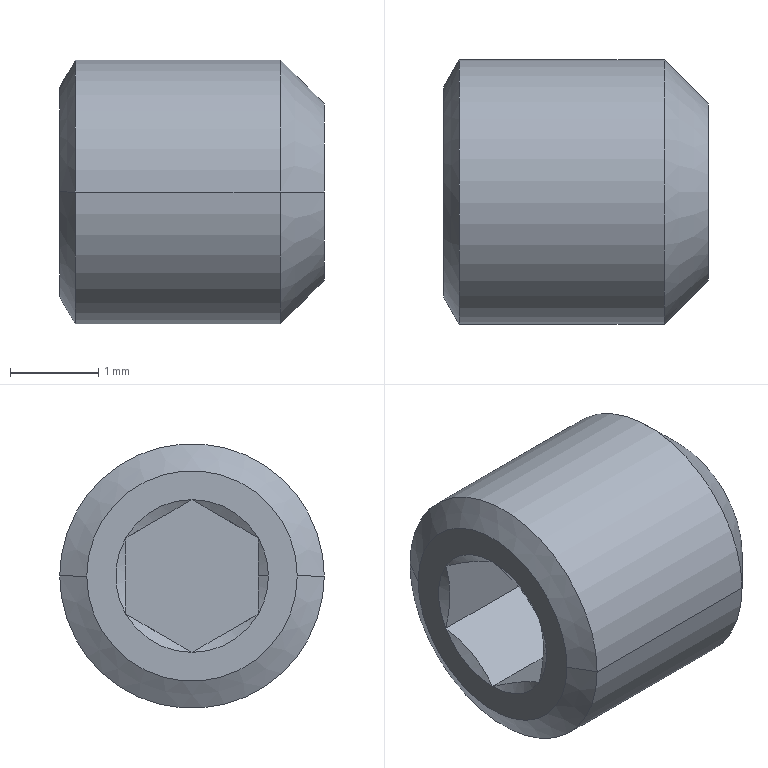Part | STEP file | 1 solid | 22 faces | box 3 x 3 x 3 mm | volume 17.571 mm3 | cone 11 | plane 9 | cylinder 2 | commonest cylinder face diameters 3 x2
STEP:
#1=CARTESIAN_POINT('',(0.,-1.194,0.));
#2=VERTEX_POINT('',#1);
#3=CARTESIAN_POINT('',(0.,1.194,0.));
#4=VERTEX_POINT('',#3);
#5=CARTESIAN_POINT('',(0.,0.,0.));
#6=DIRECTION('',(-1.,0.,0.));
#7=DIRECTION('',(0.,-1.,0.));
#8=AXIS2_PLACEMENT_3D('',#5,#6,#7);
#9=CIRCLE('',#8,1.194);
#10=EDGE_CURVE('',#2,#4,#9,.T.);
#11=ORIENTED_EDGE('',*,*,#10,.F.);
#12=CARTESIAN_POINT('',(0.177,-1.5,0.));
#13=VERTEX_POINT('',#12);
#14=CARTESIAN_POINT('',(0.,-1.194,0.));
#15=DIRECTION('',(0.5,-0.866,0.));
#16=VECTOR('',#15,1000.);
#17=LINE('',#14,#16);
#18=EDGE_CURVE('',#2,#13,#17,.T.);
#19=ORIENTED_EDGE('',*,*,#18,.T.);
#20=CARTESIAN_POINT('',(0.177,1.5,0.));
#21=VERTEX_POINT('',#20);
#22=CARTESIAN_POINT('',(0.177,0.,0.));
#23=DIRECTION('',(-1.,0.,0.));
#24=DIRECTION('',(0.,-1.,0.));
#25=AXIS2_PLACEMENT_3D('',#22,#23,#24);
#26=CIRCLE('',#25,1.5);
#27=EDGE_CURVE('',#13,#21,#26,.T.);
#28=ORIENTED_EDGE('',*,*,#27,.T.);
#29=CARTESIAN_POINT('',(0.,1.194,0.));
#30=DIRECTION('',(0.5,0.866,0.));
#31=VECTOR('',#30,1000.);
#32=LINE('',#29,#31);
#33=EDGE_CURVE('',#4,#21,#32,.T.);
#34=ORIENTED_EDGE('',*,*,#33,.F.);
#35=EDGE_LOOP('',(#11,#19,#28,#34));
#36=FACE_OUTER_BOUND('',#35,.T.);
#37=CARTESIAN_POINT('',(0.,0.,0.));
#38=DIRECTION('',(1.,0.,0.));
#39=DIRECTION('',(0.,1.,0.));
#40=AXIS2_PLACEMENT_3D('',#37,#38,#39);
#41=CONICAL_SURFACE('',#40,1.194,1.047);
#42=ADVANCED_FACE('',(#36),#41,.T.);
#43=CARTESIAN_POINT('',(2.5,-1.5,0.));
#44=VERTEX_POINT('',#43);
#45=CARTESIAN_POINT('',(2.5,1.5,0.));
#46=VERTEX_POINT('',#45);
#47=CARTESIAN_POINT('',(2.5,0.,0.));
#48=DIRECTION('',(-1.,0.,0.));
#49=DIRECTION('',(0.,-1.,0.));
#50=AXIS2_PLACEMENT_3D('',#47,#48,#49);
#51=CIRCLE('',#50,1.5);
#52=EDGE_CURVE('',#44,#46,#51,.T.);
#53=ORIENTED_EDGE('',*,*,#52,.T.);
#54=CARTESIAN_POINT('',(0.5,1.5,0.));
#55=DIRECTION('',(-1.,0.,0.));
#56=VECTOR('',#55,1000.);
#57=LINE('',#54,#56);
#58=EDGE_CURVE('',#46,#21,#57,.T.);
#59=ORIENTED_EDGE('',*,*,#58,.T.);
#60=ORIENTED_EDGE('',*,*,#27,.F.);
#61=CARTESIAN_POINT('',(0.5,-1.5,0.));
#62=DIRECTION('',(-1.,0.,0.));
#63=VECTOR('',#62,1000.);
#64=LINE('',#61,#63);
#65=EDGE_CURVE('',#44,#13,#64,.T.);
#66=ORIENTED_EDGE('',*,*,#65,.F.);
#67=EDGE_LOOP('',(#53,#59,#60,#66));
#68=FACE_OUTER_BOUND('',#67,.T.);
#69=CARTESIAN_POINT('',(0.5,0.,0.));
#70=DIRECTION('',(-1.,0.,0.));
#71=DIRECTION('',(0.,-1.,0.));
#72=AXIS2_PLACEMENT_3D('',#69,#70,#71);
#73=CYLINDRICAL_SURFACE('',#72,1.5);
#74=ADVANCED_FACE('',(#68),#73,.T.);
#75=CARTESIAN_POINT('',(3.,-1.,0.));
#76=VERTEX_POINT('',#75);
#77=CARTESIAN_POINT('',(3.,1.,0.));
#78=VERTEX_POINT('',#77);
#79=CARTESIAN_POINT('',(3.,0.,0.));
#80=DIRECTION('',(-1.,0.,0.));
#81=DIRECTION('',(0.,-1.,0.));
#82=AXIS2_PLACEMENT_3D('',#79,#80,#81);
#83=CIRCLE('',#82,1.);
#84=EDGE_CURVE('',#76,#78,#83,.T.);
#85=ORIENTED_EDGE('',*,*,#84,.T.);
#86=CARTESIAN_POINT('',(2.5,1.5,0.));
#87=DIRECTION('',(-0.7071,0.7071,0.));
#88=VECTOR('',#87,1000.);
#89=LINE('',#86,#88);
#90=EDGE_CURVE('',#78,#46,#89,.T.);
#91=ORIENTED_EDGE('',*,*,#90,.T.);
#92=ORIENTED_EDGE('',*,*,#52,.F.);
#93=CARTESIAN_POINT('',(2.5,-1.5,0.));
#94=DIRECTION('',(-0.7071,-0.7071,0.));
#95=VECTOR('',#94,1000.);
#96=LINE('',#93,#95);
#97=EDGE_CURVE('',#76,#44,#96,.T.);
#98=ORIENTED_EDGE('',*,*,#97,.F.);
#99=EDGE_LOOP('',(#85,#91,#92,#98));
#100=FACE_OUTER_BOUND('',#99,.T.);
#101=CARTESIAN_POINT('',(2.5,0.,0.));
#102=DIRECTION('',(-1.,0.,0.));
#103=DIRECTION('',(0.,-1.,0.));
#104=AXIS2_PLACEMENT_3D('',#101,#102,#103);
#105=CONICAL_SURFACE('',#104,1.5,0.7854);
#106=ADVANCED_FACE('',(#100),#105,.T.);
#107=CARTESIAN_POINT('',(0.,-0.75,0.433));
#108=VERTEX_POINT('',#107);
#109=CARTESIAN_POINT('',(0.06699,-0.75,0.));
#110=VERTEX_POINT('',#109);
#111=CARTESIAN_POINT('',(0.,-0.75,0.433));
#112=CARTESIAN_POINT('',(0.04042,-0.75,0.293));
#113=CARTESIAN_POINT('',(0.06699,-0.75,0.1463));
#114=CARTESIAN_POINT('',(0.06699,-0.75,0.));
#115=B_SPLINE_CURVE_WITH_KNOTS('',3,(#111,#112,#113,#114),.UNSPECIFIED.,.F.,.F.,(4,4),(0.002319,0.002758),.UNSPECIFIED.);
#116=EDGE_CURVE('',#108,#110,#115,.T.);
#117=ORIENTED_EDGE('',*,*,#116,.T.);
#118=CARTESIAN_POINT('',(0.,-0.866,0.));
#119=VERTEX_POINT('',#118);
#120=CARTESIAN_POINT('',(0.5,0.,0.));
#121=DIRECTION('',(-0.5,-0.866,0.));
#122=VECTOR('',#121,1000.);
#123=LINE('',#120,#122);
#124=EDGE_CURVE('',#110,#119,#123,.T.);
#125=ORIENTED_EDGE('',*,*,#124,.T.);
#126=CARTESIAN_POINT('',(0.,0.,0.));
#127=DIRECTION('',(-1.,0.,0.));
#128=DIRECTION('',(0.,-1.,0.));
#129=AXIS2_PLACEMENT_3D('',#126,#127,#128);
#130=CIRCLE('',#129,0.866);
#131=EDGE_CURVE('',#119,#108,#130,.T.);
#132=ORIENTED_EDGE('',*,*,#131,.T.);
#133=EDGE_LOOP('',(#117,#125,#132));
#134=FACE_OUTER_BOUND('',#133,.T.);
#135=CARTESIAN_POINT('',(-999.5,0.,0.));
#136=DIRECTION('',(-1.,0.,0.));
#137=DIRECTION('',(0.,-1.,0.));
#138=AXIS2_PLACEMENT_3D('',#135,#136,#137);
#139=CONICAL_SURFACE('',#138,1732.051,1.047);
#140=ADVANCED_FACE('',(#134),#139,.F.);
#141=CARTESIAN_POINT('',(0.,0.,0.866));
#142=VERTEX_POINT('',#141);
#143=CARTESIAN_POINT('',(0.,0.75,0.433));
#144=VERTEX_POINT('',#143);
#145=CARTESIAN_POINT('',(0.,0.,0.));
#146=DIRECTION('',(-1.,0.,0.));
#147=DIRECTION('',(0.,-1.,0.));
#148=AXIS2_PLACEMENT_3D('',#145,#146,#147);
#149=CIRCLE('',#148,0.866);
#150=EDGE_CURVE('',#142,#144,#149,.T.);
#151=ORIENTED_EDGE('',*,*,#150,.T.);
#152=CARTESIAN_POINT('',(0.,0.75,0.433));
#153=CARTESIAN_POINT('',(0.04082,0.6275,0.5037));
#154=CARTESIAN_POINT('',(0.06689,0.5032,0.5755));
#155=CARTESIAN_POINT('',(0.06708,0.2482,0.7227));
#156=CARTESIAN_POINT('',(0.04087,0.1226,0.7952));
#157=CARTESIAN_POINT('',(0.,0.,0.866));
#158=B_SPLINE_CURVE_WITH_KNOTS('',3,(#152,#153,#154,#155,#156,#157),.UNSPECIFIED.,.F.,.F.,(4,2,4),(0.000000238,0.0004376,0.0008749),.UNSPECIFIED.);
#159=EDGE_CURVE('',#144,#142,#158,.T.);
#160=ORIENTED_EDGE('',*,*,#159,.T.);
#161=EDGE_LOOP('',(#151,#160));
#162=FACE_OUTER_BOUND('',#161,.T.);
#163=CARTESIAN_POINT('',(-999.5,0.,0.));
#164=DIRECTION('',(-1.,0.,0.));
#165=DIRECTION('',(0.,-1.,0.));
#166=AXIS2_PLACEMENT_3D('',#163,#164,#165);
#167=CONICAL_SURFACE('',#166,1732.051,1.047);
#168=ADVANCED_FACE('',(#162),#167,.F.);
#169=CARTESIAN_POINT('',(0.,0.,0.));
#170=DIRECTION('',(-1.,0.,0.));
#171=DIRECTION('',(0.,-1.,0.));
#172=AXIS2_PLACEMENT_3D('',#169,#170,#171);
#173=CIRCLE('',#172,0.866);
#174=EDGE_CURVE('',#108,#142,#173,.T.);
#175=ORIENTED_EDGE('',*,*,#174,.T.);
#176=CARTESIAN_POINT('',(0.,0.,0.866));
#177=CARTESIAN_POINT('',(0.04082,-0.1225,0.7953));
#178=CARTESIAN_POINT('',(0.06689,-0.2468,0.7236));
#179=CARTESIAN_POINT('',(0.06708,-0.5018,0.5763));
#180=CARTESIAN_POINT('',(0.04087,-0.6274,0.5038));
#181=CARTESIAN_POINT('',(0.,-0.75,0.433));
#182=B_SPLINE_CURVE_WITH_KNOTS('',3,(#176,#177,#178,#179,#180,#181),.UNSPECIFIED.,.F.,.F.,(4,2,4),(0.000000238,0.0004376,0.0008749),.UNSPECIFIED.);
#183=EDGE_CURVE('',#142,#108,#182,.T.);
#184=ORIENTED_EDGE('',*,*,#183,.T.);
#185=EDGE_LOOP('',(#175,#184));
#186=FACE_OUTER_BOUND('',#185,.T.);
#187=CARTESIAN_POINT('',(-999.5,0.,0.));
#188=DIRECTION('',(-1.,0.,0.));
#189=DIRECTION('',(0.,-1.,0.));
#190=AXIS2_PLACEMENT_3D('',#187,#188,#189);
#191=CONICAL_SURFACE('',#190,1732.051,1.047);
#192=ADVANCED_FACE('',(#186),#191,.F.);
#193=ORIENTED_EDGE('',*,*,#124,.F.);
#194=CARTESIAN_POINT('',(0.,-0.75,-0.433));
#195=VERTEX_POINT('',#194);
#196=CARTESIAN_POINT('',(0.06699,-0.75,0.));
#197=CARTESIAN_POINT('',(0.06699,-0.75,-0.1462));
#198=CARTESIAN_POINT('',(0.04061,-0.75,-0.2923));
#199=CARTESIAN_POINT('',(0.,-0.75,-0.433));
#200=B_SPLINE_CURVE_WITH_KNOTS('',3,(#196,#197,#198,#199),.UNSPECIFIED.,.F.,.F.,(4,4),(0.002758,0.003196),.UNSPECIFIED.);
#201=EDGE_CURVE('',#110,#195,#200,.T.);
#202=ORIENTED_EDGE('',*,*,#201,.T.);
#203=CARTESIAN_POINT('',(0.,0.,0.));
#204=DIRECTION('',(-1.,0.,0.));
#205=DIRECTION('',(0.,-1.,0.));
#206=AXIS2_PLACEMENT_3D('',#203,#204,#205);
#207=CIRCLE('',#206,0.866);
#208=EDGE_CURVE('',#195,#119,#207,.T.);
#209=ORIENTED_EDGE('',*,*,#208,.T.);
#210=EDGE_LOOP('',(#193,#202,#209));
#211=FACE_OUTER_BOUND('',#210,.T.);
#212=CARTESIAN_POINT('',(-999.5,0.,0.));
#213=DIRECTION('',(-1.,0.,0.));
#214=DIRECTION('',(0.,-1.,0.));
#215=AXIS2_PLACEMENT_3D('',#212,#213,#214);
#216=CONICAL_SURFACE('',#215,1732.051,1.047);
#217=ADVANCED_FACE('',(#211),#216,.F.);
#218=CARTESIAN_POINT('',(0.,0.,-0.866));
#219=VERTEX_POINT('',#218);
#220=CARTESIAN_POINT('',(0.,0.,0.));
#221=DIRECTION('',(-1.,0.,0.));
#222=DIRECTION('',(0.,-1.,0.));
#223=AXIS2_PLACEMENT_3D('',#220,#221,#222);
#224=CIRCLE('',#223,0.866);
#225=EDGE_CURVE('',#219,#195,#224,.T.);
#226=ORIENTED_EDGE('',*,*,#225,.T.);
#227=CARTESIAN_POINT('',(0.,-0.75,-0.433));
#228=CARTESIAN_POINT('',(0.04082,-0.6275,-0.5037));
#229=CARTESIAN_POINT('',(0.06689,-0.5032,-0.5755));
#230=CARTESIAN_POINT('',(0.06708,-0.2482,-0.7227));
#231=CARTESIAN_POINT('',(0.04087,-0.1226,-0.7952));
#232=CARTESIAN_POINT('',(0.,0.,-0.866));
#233=B_SPLINE_CURVE_WITH_KNOTS('',3,(#227,#228,#229,#230,#231,#232),.UNSPECIFIED.,.F.,.F.,(4,2,4),(0.000000238,0.0004376,0.0008749),.UNSPECIFIED.);
#234=EDGE_CURVE('',#195,#219,#233,.T.);
#235=ORIENTED_EDGE('',*,*,#234,.T.);
#236=EDGE_LOOP('',(#226,#235));
#237=FACE_OUTER_BOUND('',#236,.T.);
#238=CARTESIAN_POINT('',(-999.5,0.,0.));
#239=DIRECTION('',(-1.,0.,0.));
#240=DIRECTION('',(0.,-1.,0.));
#241=AXIS2_PLACEMENT_3D('',#238,#239,#240);
#242=CONICAL_SURFACE('',#241,1732.051,1.047);
#243=ADVANCED_FACE('',(#237),#242,.F.);
#244=CARTESIAN_POINT('',(0.,0.75,-0.433));
#245=VERTEX_POINT('',#244);
#246=CARTESIAN_POINT('',(0.,0.,0.));
#247=DIRECTION('',(-1.,0.,0.));
#248=DIRECTION('',(0.,-1.,0.));
#249=AXIS2_PLACEMENT_3D('',#246,#247,#248);
#250=CIRCLE('',#249,0.866);
#251=EDGE_CURVE('',#245,#219,#250,.T.);
#252=ORIENTED_EDGE('',*,*,#251,.T.);
#253=CARTESIAN_POINT('',(0.,0.,-0.866));
#254=CARTESIAN_POINT('',(0.04082,0.1225,-0.7953));
#255=CARTESIAN_POINT('',(0.06689,0.2468,-0.7236));
#256=CARTESIAN_POINT('',(0.06708,0.5018,-0.5763));
#257=CARTESIAN_POINT('',(0.04087,0.6274,-0.5038));
#258=CARTESIAN_POINT('',(0.,0.75,-0.433));
#259=B_SPLINE_CURVE_WITH_KNOTS('',3,(#253,#254,#255,#256,#257,#258),.UNSPECIFIED.,.F.,.F.,(4,2,4),(0.000000238,0.0004376,0.0008749),.UNSPECIFIED.);
#260=EDGE_CURVE('',#219,#245,#259,.T.);
#261=ORIENTED_EDGE('',*,*,#260,.T.);
#262=EDGE_LOOP('',(#252,#261));
#263=FACE_OUTER_BOUND('',#262,.T.);
#264=CARTESIAN_POINT('',(-999.5,0.,0.));
#265=DIRECTION('',(-1.,0.,0.));
#266=DIRECTION('',(0.,-1.,0.));
#267=AXIS2_PLACEMENT_3D('',#264,#265,#266);
#268=CONICAL_SURFACE('',#267,1732.051,1.047);
#269=ADVANCED_FACE('',(#263),#268,.F.);
#270=CARTESIAN_POINT('',(0.,0.,0.));
#271=DIRECTION('',(-1.,0.,0.));
#272=DIRECTION('',(0.,-1.,0.));
#273=AXIS2_PLACEMENT_3D('',#270,#271,#272);
#274=CIRCLE('',#273,0.866);
#275=EDGE_CURVE('',#144,#245,#274,.T.);
#276=ORIENTED_EDGE('',*,*,#275,.T.);
#277=CARTESIAN_POINT('',(0.,0.75,-0.433));
#278=CARTESIAN_POINT('',(0.04062,0.75,-0.2923));
#279=CARTESIAN_POINT('',(0.067,0.75,-0.1461));
#280=CARTESIAN_POINT('',(0.06698,0.75,0.1463));
#281=CARTESIAN_POINT('',(0.04041,0.75,0.293));
#282=CARTESIAN_POINT('',(0.,0.75,0.433));
#283=B_SPLINE_CURVE_WITH_KNOTS('',3,(#277,#278,#279,#280,#281,#282),.UNSPECIFIED.,.F.,.F.,(4,2,4),(0.0007425,0.00118,0.001618),.UNSPECIFIED.);
#284=EDGE_CURVE('',#245,#144,#283,.T.);
#285=ORIENTED_EDGE('',*,*,#284,.T.);
#286=EDGE_LOOP('',(#276,#285));
#287=FACE_OUTER_BOUND('',#286,.T.);
#288=CARTESIAN_POINT('',(-999.5,0.,0.));
#289=DIRECTION('',(-1.,0.,0.));
#290=DIRECTION('',(0.,-1.,0.));
#291=AXIS2_PLACEMENT_3D('',#288,#289,#290);
#292=CONICAL_SURFACE('',#291,1732.051,1.047);
#293=ADVANCED_FACE('',(#287),#292,.F.);
#294=ORIENTED_EDGE('',*,*,#84,.F.);
#295=CARTESIAN_POINT('',(3.,0.,0.));
#296=DIRECTION('',(-1.,0.,0.));
#297=DIRECTION('',(0.,-1.,0.));
#298=AXIS2_PLACEMENT_3D('',#295,#296,#297);
#299=CIRCLE('',#298,1.);
#300=EDGE_CURVE('',#78,#76,#299,.T.);
#301=ORIENTED_EDGE('',*,*,#300,.F.);
#302=EDGE_LOOP('',(#294,#301));
#303=FACE_OUTER_BOUND('',#302,.T.);
#304=CARTESIAN_POINT('',(3.,0.,0.));
#305=DIRECTION('',(1.,0.,0.));
#306=DIRECTION('',(0.,1.,0.));
#307=AXIS2_PLACEMENT_3D('',#304,#305,#306);
#308=PLANE('',#307);
#309=ADVANCED_FACE('',(#303),#308,.T.);
#310=ORIENTED_EDGE('',*,*,#90,.F.);
#311=ORIENTED_EDGE('',*,*,#300,.T.);
#312=ORIENTED_EDGE('',*,*,#97,.T.);
#313=CARTESIAN_POINT('',(2.5,0.,0.));
#314=DIRECTION('',(-1.,0.,0.));
#315=DIRECTION('',(0.,-1.,0.));
#316=AXIS2_PLACEMENT_3D('',#313,#314,#315);
#317=CIRCLE('',#316,1.5);
#318=EDGE_CURVE('',#46,#44,#317,.T.);
#319=ORIENTED_EDGE('',*,*,#318,.F.);
#320=EDGE_LOOP('',(#310,#311,#312,#319));
#321=FACE_OUTER_BOUND('',#320,.T.);
#322=CARTESIAN_POINT('',(2.5,0.,0.));
#323=DIRECTION('',(-1.,0.,0.));
#324=DIRECTION('',(0.,-1.,0.));
#325=AXIS2_PLACEMENT_3D('',#322,#323,#324);
#326=CONICAL_SURFACE('',#325,1.5,0.7854);
#327=ADVANCED_FACE('',(#321),#326,.T.);
#328=ORIENTED_EDGE('',*,*,#58,.F.);
#329=ORIENTED_EDGE('',*,*,#318,.T.);
#330=ORIENTED_EDGE('',*,*,#65,.T.);
#331=CARTESIAN_POINT('',(0.177,0.,0.));
#332=DIRECTION('',(-1.,0.,0.));
#333=DIRECTION('',(0.,-1.,0.));
#334=AXIS2_PLACEMENT_3D('',#331,#332,#333);
#335=CIRCLE('',#334,1.5);
#336=EDGE_CURVE('',#21,#13,#335,.T.);
#337=ORIENTED_EDGE('',*,*,#336,.F.);
#338=EDGE_LOOP('',(#328,#329,#330,#337));
#339=FACE_OUTER_BOUND('',#338,.T.);
#340=CARTESIAN_POINT('',(0.5,0.,0.));
#341=DIRECTION('',(-1.,0.,0.));
#342=DIRECTION('',(0.,-1.,0.));
#343=AXIS2_PLACEMENT_3D('',#340,#341,#342);
#344=CYLINDRICAL_SURFACE('',#343,1.5);
#345=ADVANCED_FACE('',(#339),#344,.T.);
#346=ORIENTED_EDGE('',*,*,#18,.F.);
#347=CARTESIAN_POINT('',(0.,0.,0.));
#348=DIRECTION('',(-1.,0.,0.));
#349=DIRECTION('',(0.,-1.,0.));
#350=AXIS2_PLACEMENT_3D('',#347,#348,#349);
#351=CIRCLE('',#350,1.194);
#352=EDGE_CURVE('',#4,#2,#351,.T.);
#353=ORIENTED_EDGE('',*,*,#352,.F.);
#354=ORIENTED_EDGE('',*,*,#33,.T.);
#355=ORIENTED_EDGE('',*,*,#336,.T.);
#356=EDGE_LOOP('',(#346,#353,#354,#355));
#357=FACE_OUTER_BOUND('',#356,.T.);
#358=CARTESIAN_POINT('',(0.,0.,0.));
#359=DIRECTION('',(1.,0.,0.));
#360=DIRECTION('',(0.,1.,0.));
#361=AXIS2_PLACEMENT_3D('',#358,#359,#360);
#362=CONICAL_SURFACE('',#361,1.194,1.047);
#363=ADVANCED_FACE('',(#357),#362,.T.);
#364=ORIENTED_EDGE('',*,*,#352,.T.);
#365=ORIENTED_EDGE('',*,*,#10,.T.);
#366=EDGE_LOOP('',(#364,#365));
#367=FACE_OUTER_BOUND('',#366,.T.);
#368=ORIENTED_EDGE('',*,*,#174,.F.);
#369=ORIENTED_EDGE('',*,*,#131,.F.);
#370=ORIENTED_EDGE('',*,*,#208,.F.);
#371=ORIENTED_EDGE('',*,*,#225,.F.);
#372=ORIENTED_EDGE('',*,*,#251,.F.);
#373=ORIENTED_EDGE('',*,*,#275,.F.);
#374=ORIENTED_EDGE('',*,*,#150,.F.);
#375=EDGE_LOOP('',(#368,#369,#370,#371,#372,#373,#374));
#376=FACE_BOUND('',#375,.T.);
#377=CARTESIAN_POINT('',(0.,-1.194,0.));
#378=DIRECTION('',(-1.,0.,0.));
#379=DIRECTION('',(0.,-1.,0.));
#380=AXIS2_PLACEMENT_3D('',#377,#378,#379);
#381=PLANE('',#380);
#382=ADVANCED_FACE('',(#367,#376),#381,.T.);
#383=CARTESIAN_POINT('',(1.2,0.75,0.433));
#384=VERTEX_POINT('',#383);
#385=CARTESIAN_POINT('',(1.2,0.75,0.433));
#386=DIRECTION('',(-1.,0.,0.));
#387=VECTOR('',#386,1000.);
#388=LINE('',#385,#387);
#389=EDGE_CURVE('',#384,#144,#388,.T.);
#390=ORIENTED_EDGE('',*,*,#389,.F.);
#391=CARTESIAN_POINT('',(1.2,0.,0.866));
#392=VERTEX_POINT('',#391);
#393=CARTESIAN_POINT('',(1.2,0.75,0.433));
#394=DIRECTION('',(0.,-0.866,0.5));
#395=VECTOR('',#394,1000.);
#396=LINE('',#393,#395);
#397=EDGE_CURVE('',#384,#392,#396,.T.);
#398=ORIENTED_EDGE('',*,*,#397,.T.);
#399=CARTESIAN_POINT('',(1.2,0.,0.866));
#400=DIRECTION('',(-1.,0.,0.));
#401=VECTOR('',#400,1000.);
#402=LINE('',#399,#401);
#403=EDGE_CURVE('',#392,#142,#402,.T.);
#404=ORIENTED_EDGE('',*,*,#403,.T.);
#405=ORIENTED_EDGE('',*,*,#159,.F.);
#406=EDGE_LOOP('',(#390,#398,#404,#405));
#407=FACE_OUTER_BOUND('',#406,.T.);
#408=CARTESIAN_POINT('',(1.2,0.75,0.433));
#409=DIRECTION('',(0.,-0.5,-0.866));
#410=DIRECTION('',(0.,0.866,-0.5));
#411=AXIS2_PLACEMENT_3D('',#408,#409,#410);
#412=PLANE('',#411);
#413=ADVANCED_FACE('',(#407),#412,.T.);
#414=ORIENTED_EDGE('',*,*,#403,.F.);
#415=CARTESIAN_POINT('',(1.2,-0.75,0.433));
#416=VERTEX_POINT('',#415);
#417=CARTESIAN_POINT('',(1.2,0.,0.866));
#418=DIRECTION('',(0.,-0.866,-0.5));
#419=VECTOR('',#418,1000.);
#420=LINE('',#417,#419);
#421=EDGE_CURVE('',#392,#416,#420,.T.);
#422=ORIENTED_EDGE('',*,*,#421,.T.);
#423=CARTESIAN_POINT('',(1.2,-0.75,0.433));
#424=DIRECTION('',(-1.,0.,0.));
#425=VECTOR('',#424,1000.);
#426=LINE('',#423,#425);
#427=EDGE_CURVE('',#416,#108,#426,.T.);
#428=ORIENTED_EDGE('',*,*,#427,.T.);
#429=ORIENTED_EDGE('',*,*,#183,.F.);
#430=EDGE_LOOP('',(#414,#422,#428,#429));
#431=FACE_OUTER_BOUND('',#430,.T.);
#432=CARTESIAN_POINT('',(1.2,0.,0.866));
#433=DIRECTION('',(0.,0.5,-0.866));
#434=DIRECTION('',(0.,0.866,0.5));
#435=AXIS2_PLACEMENT_3D('',#432,#433,#434);
#436=PLANE('',#435);
#437=ADVANCED_FACE('',(#431),#436,.T.);
#438=ORIENTED_EDGE('',*,*,#427,.F.);
#439=CARTESIAN_POINT('',(1.2,-0.75,-0.433));
#440=VERTEX_POINT('',#439);
#441=CARTESIAN_POINT('',(1.2,-0.75,0.433));
#442=DIRECTION('',(0.,0.,-1.));
#443=VECTOR('',#442,1000.);
#444=LINE('',#441,#443);
#445=EDGE_CURVE('',#416,#440,#444,.T.);
#446=ORIENTED_EDGE('',*,*,#445,.T.);
#447=CARTESIAN_POINT('',(1.2,-0.75,-0.433));
#448=DIRECTION('',(-1.,0.,0.));
#449=VECTOR('',#448,1000.);
#450=LINE('',#447,#449);
#451=EDGE_CURVE('',#440,#195,#450,.T.);
#452=ORIENTED_EDGE('',*,*,#451,.T.);
#453=ORIENTED_EDGE('',*,*,#201,.F.);
#454=ORIENTED_EDGE('',*,*,#116,.F.);
#455=EDGE_LOOP('',(#438,#446,#452,#453,#454));
#456=FACE_OUTER_BOUND('',#455,.T.);
#457=CARTESIAN_POINT('',(1.2,-0.75,0.433));
#458=DIRECTION('',(0.,1.,0.));
#459=DIRECTION('',(0.,0.,1.));
#460=AXIS2_PLACEMENT_3D('',#457,#458,#459);
#461=PLANE('',#460);
#462=ADVANCED_FACE('',(#456),#461,.T.);
#463=ORIENTED_EDGE('',*,*,#451,.F.);
#464=CARTESIAN_POINT('',(1.2,0.,-0.866));
#465=VERTEX_POINT('',#464);
#466=CARTESIAN_POINT('',(1.2,-0.75,-0.433));
#467=DIRECTION('',(0.,0.866,-0.5));
#468=VECTOR('',#467,1000.);
#469=LINE('',#466,#468);
#470=EDGE_CURVE('',#440,#465,#469,.T.);
#471=ORIENTED_EDGE('',*,*,#470,.T.);
#472=CARTESIAN_POINT('',(1.2,0.,-0.866));
#473=DIRECTION('',(-1.,0.,0.));
#474=VECTOR('',#473,1000.);
#475=LINE('',#472,#474);
#476=EDGE_CURVE('',#465,#219,#475,.T.);
#477=ORIENTED_EDGE('',*,*,#476,.T.);
#478=ORIENTED_EDGE('',*,*,#234,.F.);
#479=EDGE_LOOP('',(#463,#471,#477,#478));
#480=FACE_OUTER_BOUND('',#479,.T.);
#481=CARTESIAN_POINT('',(1.2,-0.75,-0.433));
#482=DIRECTION('',(0.,0.5,0.866));
#483=DIRECTION('',(0.,-0.866,0.5));
#484=AXIS2_PLACEMENT_3D('',#481,#482,#483);
#485=PLANE('',#484);
#486=ADVANCED_FACE('',(#480),#485,.T.);
#487=ORIENTED_EDGE('',*,*,#476,.F.);
#488=CARTESIAN_POINT('',(1.2,0.75,-0.433));
#489=VERTEX_POINT('',#488);
#490=CARTESIAN_POINT('',(1.2,0.,-0.866));
#491=DIRECTION('',(0.,0.866,0.5));
#492=VECTOR('',#491,1000.);
#493=LINE('',#490,#492);
#494=EDGE_CURVE('',#465,#489,#493,.T.);
#495=ORIENTED_EDGE('',*,*,#494,.T.);
#496=CARTESIAN_POINT('',(1.2,0.75,-0.433));
#497=DIRECTION('',(-1.,0.,0.));
#498=VECTOR('',#497,1000.);
#499=LINE('',#496,#498);
#500=EDGE_CURVE('',#489,#245,#499,.T.);
#501=ORIENTED_EDGE('',*,*,#500,.T.);
#502=ORIENTED_EDGE('',*,*,#260,.F.);
#503=EDGE_LOOP('',(#487,#495,#501,#502));
#504=FACE_OUTER_BOUND('',#503,.T.);
#505=CARTESIAN_POINT('',(1.2,0.,-0.866));
#506=DIRECTION('',(0.,-0.5,0.866));
#507=DIRECTION('',(0.,-0.866,-0.5));
#508=AXIS2_PLACEMENT_3D('',#505,#506,#507);
#509=PLANE('',#508);
#510=ADVANCED_FACE('',(#504),#509,.T.);
#511=ORIENTED_EDGE('',*,*,#500,.F.);
#512=CARTESIAN_POINT('',(1.2,0.75,-0.433));
#513=DIRECTION('',(0.,0.,1.));
#514=VECTOR('',#513,1000.);
#515=LINE('',#512,#514);
#516=EDGE_CURVE('',#489,#384,#515,.T.);
#517=ORIENTED_EDGE('',*,*,#516,.T.);
#518=ORIENTED_EDGE('',*,*,#389,.T.);
#519=ORIENTED_EDGE('',*,*,#284,.F.);
#520=EDGE_LOOP('',(#511,#517,#518,#519));
#521=FACE_OUTER_BOUND('',#520,.T.);
#522=CARTESIAN_POINT('',(1.2,0.75,-0.433));
#523=DIRECTION('',(0.,-1.,0.));
#524=DIRECTION('',(0.,0.,-1.));
#525=AXIS2_PLACEMENT_3D('',#522,#523,#524);
#526=PLANE('',#525);
#527=ADVANCED_FACE('',(#521),#526,.T.);
#528=ORIENTED_EDGE('',*,*,#397,.F.);
#529=ORIENTED_EDGE('',*,*,#516,.F.);
#530=ORIENTED_EDGE('',*,*,#494,.F.);
#531=ORIENTED_EDGE('',*,*,#470,.F.);
#532=ORIENTED_EDGE('',*,*,#445,.F.);
#533=ORIENTED_EDGE('',*,*,#421,.F.);
#534=EDGE_LOOP('',(#528,#529,#530,#531,#532,#533));
#535=FACE_OUTER_BOUND('',#534,.T.);
#536=CARTESIAN_POINT('',(1.2,0.,0.));
#537=DIRECTION('',(1.,0.,0.));
#538=DIRECTION('',(0.,0.,-1.));
#539=AXIS2_PLACEMENT_3D('',#536,#537,#538);
#540=PLANE('',#539);
#541=ADVANCED_FACE('',(#535),#540,.F.);
#542=CLOSED_SHELL('',(#42,#74,#106,#140,#168,#192,#217,#243,#269,#293,#309,#327,#345,#363,#382,#413,#437,#462,#486,#510,#527,#541));
#543=MANIFOLD_SOLID_BREP('',#542);
#544=CARTESIAN_POINT('',(0.,0.,0.));
#545=DIRECTION('',(0.,0.,1.));
#546=DIRECTION('',(1.,0.,0.));
#547=AXIS2_PLACEMENT_3D('',#544,#545,#546);
#548=(LENGTH_UNIT()NAMED_UNIT(*)SI_UNIT(.MILLI.,.METRE.));
#549=UNCERTAINTY_MEASURE_WITH_UNIT(LENGTH_MEASURE(0.00001),#548,'','');
#550=(NAMED_UNIT(*)PLANE_ANGLE_UNIT()SI_UNIT($,.RADIAN.));
#551=(NAMED_UNIT(*)SI_UNIT($,.STERADIAN.)SOLID_ANGLE_UNIT());
#552=(GEOMETRIC_REPRESENTATION_CONTEXT(3)GLOBAL_UNCERTAINTY_ASSIGNED_CONTEXT((#549))GLOBAL_UNIT_ASSIGNED_CONTEXT((#548,#550,#551))REPRESENTATION_CONTEXT('',''));
#553=ADVANCED_BREP_SHAPE_REPRESENTATION('',(#543,#547),#552);